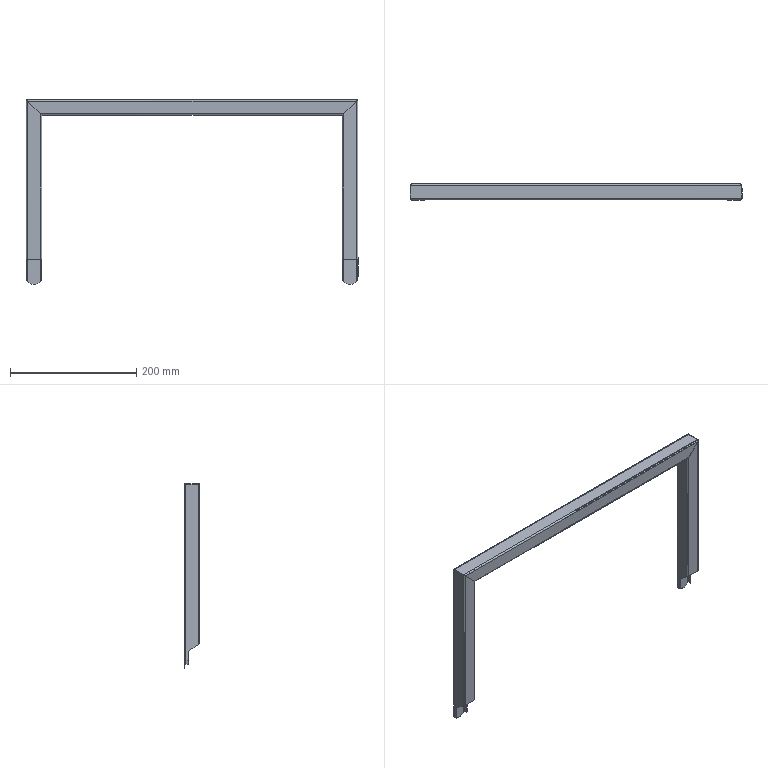Part | SolidWorks | features Fillet 2, ICE 2, WeldMemberFeat 1, WeldmentFeature 1 | 3 solids | 64 faces | box 525 x 25 x 292.5 mm | volume 111905 mm3 | plane 36 | cylinder 28 | commonest cylinder face diameters 2.4 x12 4.8 x12 24 x4